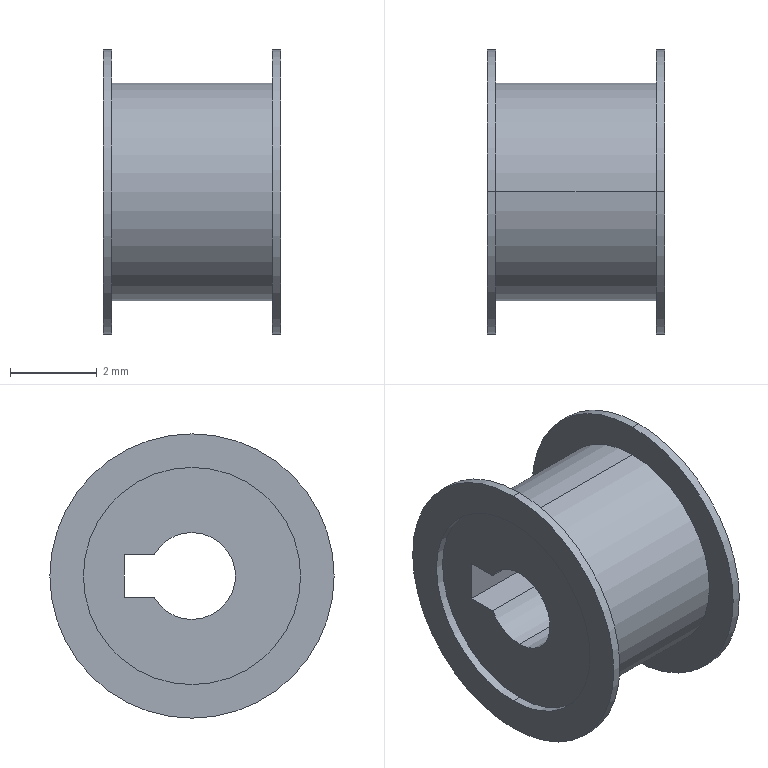Part | SolidWorks | features ICE 1, Revolution 1 | 3 solids | 22 faces | box 4.086 x 6.543 x 6.543 mm | volume 64.18 mm3 | cylinder 13 | plane 9 | commonest cylinder face diameters 5 x6 6.543 x4 2 x3
STEP:
#1=CARTESIAN_POINT('',(2.043,0.,3.271));
#2=VERTEX_POINT('',#1);
#3=CARTESIAN_POINT('',(2.043,0.,-3.271));
#4=VERTEX_POINT('',#3);
#5=CARTESIAN_POINT('',(2.043,0.,0.));
#6=DIRECTION('',(-1.,0.,0.));
#7=DIRECTION('',(0.,0.,1.));
#8=AXIS2_PLACEMENT_3D('',#5,#6,#7);
#9=CIRCLE('',#8,3.271);
#10=EDGE_CURVE('',#2,#4,#9,.T.);
#11=ORIENTED_EDGE('',*,*,#10,.T.);
#12=CARTESIAN_POINT('',(1.843,0.,-3.271));
#13=VERTEX_POINT('',#12);
#14=CARTESIAN_POINT('',(0.,0.,-3.271));
#15=DIRECTION('',(-1.,0.,0.));
#16=VECTOR('',#15,1000.);
#17=LINE('',#14,#16);
#18=EDGE_CURVE('',#4,#13,#17,.T.);
#19=ORIENTED_EDGE('',*,*,#18,.T.);
#20=CARTESIAN_POINT('',(1.843,0.,3.271));
#21=VERTEX_POINT('',#20);
#22=CARTESIAN_POINT('',(1.843,0.,0.));
#23=DIRECTION('',(-1.,0.,0.));
#24=DIRECTION('',(0.,0.,1.));
#25=AXIS2_PLACEMENT_3D('',#22,#23,#24);
#26=CIRCLE('',#25,3.271);
#27=EDGE_CURVE('',#21,#13,#26,.T.);
#28=ORIENTED_EDGE('',*,*,#27,.F.);
#29=CARTESIAN_POINT('',(0.,0.,3.271));
#30=DIRECTION('',(-1.,0.,0.));
#31=VECTOR('',#30,1000.);
#32=LINE('',#29,#31);
#33=EDGE_CURVE('',#2,#21,#32,.T.);
#34=ORIENTED_EDGE('',*,*,#33,.F.);
#35=EDGE_LOOP('',(#11,#19,#28,#34));
#36=FACE_OUTER_BOUND('',#35,.T.);
#37=CARTESIAN_POINT('',(0.,0.,0.));
#38=DIRECTION('',(-1.,0.,0.));
#39=DIRECTION('',(0.,0.,1.));
#40=AXIS2_PLACEMENT_3D('',#37,#38,#39);
#41=CYLINDRICAL_SURFACE('',#40,3.271);
#42=ADVANCED_FACE('',(#36),#41,.T.);
#43=CARTESIAN_POINT('',(2.043,0.,-2.5));
#44=VERTEX_POINT('',#43);
#45=CARTESIAN_POINT('',(2.043,0.,2.5));
#46=VERTEX_POINT('',#45);
#47=CARTESIAN_POINT('',(2.043,0.,0.));
#48=DIRECTION('',(-1.,0.,0.));
#49=DIRECTION('',(0.,0.,1.));
#50=AXIS2_PLACEMENT_3D('',#47,#48,#49);
#51=CIRCLE('',#50,2.5);
#52=EDGE_CURVE('',#44,#46,#51,.T.);
#53=ORIENTED_EDGE('',*,*,#52,.F.);
#54=CARTESIAN_POINT('',(1.843,0.,-2.5));
#55=VERTEX_POINT('',#54);
#56=CARTESIAN_POINT('',(0.,0.,-2.5));
#57=DIRECTION('',(-1.,0.,0.));
#58=VECTOR('',#57,1000.);
#59=LINE('',#56,#58);
#60=EDGE_CURVE('',#44,#55,#59,.T.);
#61=ORIENTED_EDGE('',*,*,#60,.T.);
#62=CARTESIAN_POINT('',(1.843,0.,2.5));
#63=VERTEX_POINT('',#62);
#64=CARTESIAN_POINT('',(1.843,0.,0.));
#65=DIRECTION('',(-1.,0.,0.));
#66=DIRECTION('',(0.,0.,1.));
#67=AXIS2_PLACEMENT_3D('',#64,#65,#66);
#68=CIRCLE('',#67,2.5);
#69=EDGE_CURVE('',#55,#63,#68,.T.);
#70=ORIENTED_EDGE('',*,*,#69,.T.);
#71=CARTESIAN_POINT('',(0.,0.,2.5));
#72=DIRECTION('',(-1.,0.,0.));
#73=VECTOR('',#72,1000.);
#74=LINE('',#71,#73);
#75=EDGE_CURVE('',#46,#63,#74,.T.);
#76=ORIENTED_EDGE('',*,*,#75,.F.);
#77=EDGE_LOOP('',(#53,#61,#70,#76));
#78=FACE_OUTER_BOUND('',#77,.T.);
#79=CARTESIAN_POINT('',(0.,0.,0.));
#80=DIRECTION('',(-1.,0.,0.));
#81=DIRECTION('',(0.,0.,1.));
#82=AXIS2_PLACEMENT_3D('',#79,#80,#81);
#83=CYLINDRICAL_SURFACE('',#82,2.5);
#84=ADVANCED_FACE('',(#78),#83,.F.);
#85=ORIENTED_EDGE('',*,*,#27,.T.);
#86=CARTESIAN_POINT('',(1.843,0.,0.));
#87=DIRECTION('',(-1.,0.,0.));
#88=DIRECTION('',(0.,0.,1.));
#89=AXIS2_PLACEMENT_3D('',#86,#87,#88);
#90=CIRCLE('',#89,3.271);
#91=EDGE_CURVE('',#13,#21,#90,.T.);
#92=ORIENTED_EDGE('',*,*,#91,.T.);
#93=EDGE_LOOP('',(#85,#92));
#94=FACE_OUTER_BOUND('',#93,.T.);
#95=CARTESIAN_POINT('',(1.843,0.,0.));
#96=DIRECTION('',(-1.,0.,0.));
#97=DIRECTION('',(0.,0.,1.));
#98=AXIS2_PLACEMENT_3D('',#95,#96,#97);
#99=CIRCLE('',#98,2.5);
#100=EDGE_CURVE('',#63,#55,#99,.T.);
#101=ORIENTED_EDGE('',*,*,#100,.F.);
#102=ORIENTED_EDGE('',*,*,#69,.F.);
#103=EDGE_LOOP('',(#101,#102));
#104=FACE_BOUND('',#103,.T.);
#105=CARTESIAN_POINT('',(1.843,0.,0.));
#106=DIRECTION('',(-1.,0.,0.));
#107=DIRECTION('',(0.,0.,1.));
#108=AXIS2_PLACEMENT_3D('',#105,#106,#107);
#109=PLANE('',#108);
#110=ADVANCED_FACE('',(#94,#104),#109,.T.);
#111=ORIENTED_EDGE('',*,*,#60,.F.);
#112=CARTESIAN_POINT('',(2.043,0.,0.));
#113=DIRECTION('',(-1.,0.,0.));
#114=DIRECTION('',(0.,0.,1.));
#115=AXIS2_PLACEMENT_3D('',#112,#113,#114);
#116=CIRCLE('',#115,2.5);
#117=EDGE_CURVE('',#46,#44,#116,.T.);
#118=ORIENTED_EDGE('',*,*,#117,.F.);
#119=ORIENTED_EDGE('',*,*,#75,.T.);
#120=ORIENTED_EDGE('',*,*,#100,.T.);
#121=EDGE_LOOP('',(#111,#118,#119,#120));
#122=FACE_OUTER_BOUND('',#121,.T.);
#123=CARTESIAN_POINT('',(0.,0.,0.));
#124=DIRECTION('',(-1.,0.,0.));
#125=DIRECTION('',(0.,0.,1.));
#126=AXIS2_PLACEMENT_3D('',#123,#124,#125);
#127=CYLINDRICAL_SURFACE('',#126,2.5);
#128=ADVANCED_FACE('',(#122),#127,.F.);
#129=ORIENTED_EDGE('',*,*,#10,.F.);
#130=CARTESIAN_POINT('',(2.043,0.,0.));
#131=DIRECTION('',(-1.,0.,0.));
#132=DIRECTION('',(0.,0.,1.));
#133=AXIS2_PLACEMENT_3D('',#130,#131,#132);
#134=CIRCLE('',#133,3.271);
#135=EDGE_CURVE('',#4,#2,#134,.T.);
#136=ORIENTED_EDGE('',*,*,#135,.F.);
#137=EDGE_LOOP('',(#129,#136));
#138=FACE_OUTER_BOUND('',#137,.T.);
#139=ORIENTED_EDGE('',*,*,#117,.T.);
#140=ORIENTED_EDGE('',*,*,#52,.T.);
#141=EDGE_LOOP('',(#139,#140));
#142=FACE_BOUND('',#141,.T.);
#143=CARTESIAN_POINT('',(2.043,0.,0.));
#144=DIRECTION('',(-1.,0.,0.));
#145=DIRECTION('',(0.,0.,1.));
#146=AXIS2_PLACEMENT_3D('',#143,#144,#145);
#147=PLANE('',#146);
#148=ADVANCED_FACE('',(#138,#142),#147,.F.);
#149=ORIENTED_EDGE('',*,*,#18,.F.);
#150=ORIENTED_EDGE('',*,*,#135,.T.);
#151=ORIENTED_EDGE('',*,*,#33,.T.);
#152=ORIENTED_EDGE('',*,*,#91,.F.);
#153=EDGE_LOOP('',(#149,#150,#151,#152));
#154=FACE_OUTER_BOUND('',#153,.T.);
#155=CARTESIAN_POINT('',(0.,0.,0.));
#156=DIRECTION('',(-1.,0.,0.));
#157=DIRECTION('',(0.,0.,1.));
#158=AXIS2_PLACEMENT_3D('',#155,#156,#157);
#159=CYLINDRICAL_SURFACE('',#158,3.271);
#160=ADVANCED_FACE('',(#154),#159,.T.);
#161=CLOSED_SHELL('',(#42,#84,#110,#128,#148,#160));
#162=MANIFOLD_SOLID_BREP('',#161);
#163=CARTESIAN_POINT('',(-1.843,0.,3.271));
#164=VERTEX_POINT('',#163);
#165=CARTESIAN_POINT('',(-1.843,0.,-3.271));
#166=VERTEX_POINT('',#165);
#167=CARTESIAN_POINT('',(-1.843,0.,0.));
#168=DIRECTION('',(-1.,0.,0.));
#169=DIRECTION('',(0.,0.,1.));
#170=AXIS2_PLACEMENT_3D('',#167,#168,#169);
#171=CIRCLE('',#170,3.271);
#172=EDGE_CURVE('',#164,#166,#171,.T.);
#173=ORIENTED_EDGE('',*,*,#172,.T.);
#174=CARTESIAN_POINT('',(-2.043,0.,-3.271));
#175=VERTEX_POINT('',#174);
#176=CARTESIAN_POINT('',(0.,0.,-3.271));
#177=DIRECTION('',(-1.,0.,0.));
#178=VECTOR('',#177,1000.);
#179=LINE('',#176,#178);
#180=EDGE_CURVE('',#166,#175,#179,.T.);
#181=ORIENTED_EDGE('',*,*,#180,.T.);
#182=CARTESIAN_POINT('',(-2.043,0.,3.271));
#183=VERTEX_POINT('',#182);
#184=CARTESIAN_POINT('',(-2.043,0.,0.));
#185=DIRECTION('',(-1.,0.,0.));
#186=DIRECTION('',(0.,0.,1.));
#187=AXIS2_PLACEMENT_3D('',#184,#185,#186);
#188=CIRCLE('',#187,3.271);
#189=EDGE_CURVE('',#183,#175,#188,.T.);
#190=ORIENTED_EDGE('',*,*,#189,.F.);
#191=CARTESIAN_POINT('',(0.,0.,3.271));
#192=DIRECTION('',(-1.,0.,0.));
#193=VECTOR('',#192,1000.);
#194=LINE('',#191,#193);
#195=EDGE_CURVE('',#164,#183,#194,.T.);
#196=ORIENTED_EDGE('',*,*,#195,.F.);
#197=EDGE_LOOP('',(#173,#181,#190,#196));
#198=FACE_OUTER_BOUND('',#197,.T.);
#199=CARTESIAN_POINT('',(0.,0.,0.));
#200=DIRECTION('',(-1.,0.,0.));
#201=DIRECTION('',(0.,0.,1.));
#202=AXIS2_PLACEMENT_3D('',#199,#200,#201);
#203=CYLINDRICAL_SURFACE('',#202,3.271);
#204=ADVANCED_FACE('',(#198),#203,.T.);
#205=CARTESIAN_POINT('',(-1.843,0.,-2.5));
#206=VERTEX_POINT('',#205);
#207=CARTESIAN_POINT('',(-1.843,0.,2.5));
#208=VERTEX_POINT('',#207);
#209=CARTESIAN_POINT('',(-1.843,0.,0.));
#210=DIRECTION('',(-1.,0.,0.));
#211=DIRECTION('',(0.,0.,1.));
#212=AXIS2_PLACEMENT_3D('',#209,#210,#211);
#213=CIRCLE('',#212,2.5);
#214=EDGE_CURVE('',#206,#208,#213,.T.);
#215=ORIENTED_EDGE('',*,*,#214,.F.);
#216=CARTESIAN_POINT('',(-2.043,0.,-2.5));
#217=VERTEX_POINT('',#216);
#218=CARTESIAN_POINT('',(0.,0.,-2.5));
#219=DIRECTION('',(-1.,0.,0.));
#220=VECTOR('',#219,1000.);
#221=LINE('',#218,#220);
#222=EDGE_CURVE('',#206,#217,#221,.T.);
#223=ORIENTED_EDGE('',*,*,#222,.T.);
#224=CARTESIAN_POINT('',(-2.043,0.,2.5));
#225=VERTEX_POINT('',#224);
#226=CARTESIAN_POINT('',(-2.043,0.,0.));
#227=DIRECTION('',(-1.,0.,0.));
#228=DIRECTION('',(0.,0.,1.));
#229=AXIS2_PLACEMENT_3D('',#226,#227,#228);
#230=CIRCLE('',#229,2.5);
#231=EDGE_CURVE('',#217,#225,#230,.T.);
#232=ORIENTED_EDGE('',*,*,#231,.T.);
#233=CARTESIAN_POINT('',(0.,0.,2.5));
#234=DIRECTION('',(-1.,0.,0.));
#235=VECTOR('',#234,1000.);
#236=LINE('',#233,#235);
#237=EDGE_CURVE('',#208,#225,#236,.T.);
#238=ORIENTED_EDGE('',*,*,#237,.F.);
#239=EDGE_LOOP('',(#215,#223,#232,#238));
#240=FACE_OUTER_BOUND('',#239,.T.);
#241=CARTESIAN_POINT('',(0.,0.,0.));
#242=DIRECTION('',(-1.,0.,0.));
#243=DIRECTION('',(0.,0.,1.));
#244=AXIS2_PLACEMENT_3D('',#241,#242,#243);
#245=CYLINDRICAL_SURFACE('',#244,2.5);
#246=ADVANCED_FACE('',(#240),#245,.F.);
#247=ORIENTED_EDGE('',*,*,#222,.F.);
#248=CARTESIAN_POINT('',(-1.843,0.,0.));
#249=DIRECTION('',(-1.,0.,0.));
#250=DIRECTION('',(0.,0.,1.));
#251=AXIS2_PLACEMENT_3D('',#248,#249,#250);
#252=CIRCLE('',#251,2.5);
#253=EDGE_CURVE('',#208,#206,#252,.T.);
#254=ORIENTED_EDGE('',*,*,#253,.F.);
#255=ORIENTED_EDGE('',*,*,#237,.T.);
#256=CARTESIAN_POINT('',(-2.043,0.,0.));
#257=DIRECTION('',(-1.,0.,0.));
#258=DIRECTION('',(0.,0.,1.));
#259=AXIS2_PLACEMENT_3D('',#256,#257,#258);
#260=CIRCLE('',#259,2.5);
#261=EDGE_CURVE('',#225,#217,#260,.T.);
#262=ORIENTED_EDGE('',*,*,#261,.T.);
#263=EDGE_LOOP('',(#247,#254,#255,#262));
#264=FACE_OUTER_BOUND('',#263,.T.);
#265=CARTESIAN_POINT('',(0.,0.,0.));
#266=DIRECTION('',(-1.,0.,0.));
#267=DIRECTION('',(0.,0.,1.));
#268=AXIS2_PLACEMENT_3D('',#265,#266,#267);
#269=CYLINDRICAL_SURFACE('',#268,2.5);
#270=ADVANCED_FACE('',(#264),#269,.F.);
#271=ORIENTED_EDGE('',*,*,#172,.F.);
#272=CARTESIAN_POINT('',(-1.843,0.,0.));
#273=DIRECTION('',(-1.,0.,0.));
#274=DIRECTION('',(0.,0.,1.));
#275=AXIS2_PLACEMENT_3D('',#272,#273,#274);
#276=CIRCLE('',#275,3.271);
#277=EDGE_CURVE('',#166,#164,#276,.T.);
#278=ORIENTED_EDGE('',*,*,#277,.F.);
#279=EDGE_LOOP('',(#271,#278));
#280=FACE_OUTER_BOUND('',#279,.T.);
#281=ORIENTED_EDGE('',*,*,#253,.T.);
#282=ORIENTED_EDGE('',*,*,#214,.T.);
#283=EDGE_LOOP('',(#281,#282));
#284=FACE_BOUND('',#283,.T.);
#285=CARTESIAN_POINT('',(-1.843,0.,0.));
#286=DIRECTION('',(-1.,0.,0.));
#287=DIRECTION('',(0.,0.,1.));
#288=AXIS2_PLACEMENT_3D('',#285,#286,#287);
#289=PLANE('',#288);
#290=ADVANCED_FACE('',(#280,#284),#289,.F.);
#291=ORIENTED_EDGE('',*,*,#180,.F.);
#292=ORIENTED_EDGE('',*,*,#277,.T.);
#293=ORIENTED_EDGE('',*,*,#195,.T.);
#294=CARTESIAN_POINT('',(-2.043,0.,0.));
#295=DIRECTION('',(-1.,0.,0.));
#296=DIRECTION('',(0.,0.,1.));
#297=AXIS2_PLACEMENT_3D('',#294,#295,#296);
#298=CIRCLE('',#297,3.271);
#299=EDGE_CURVE('',#175,#183,#298,.T.);
#300=ORIENTED_EDGE('',*,*,#299,.F.);
#301=EDGE_LOOP('',(#291,#292,#293,#300));
#302=FACE_OUTER_BOUND('',#301,.T.);
#303=CARTESIAN_POINT('',(0.,0.,0.));
#304=DIRECTION('',(-1.,0.,0.));
#305=DIRECTION('',(0.,0.,1.));
#306=AXIS2_PLACEMENT_3D('',#303,#304,#305);
#307=CYLINDRICAL_SURFACE('',#306,3.271);
#308=ADVANCED_FACE('',(#302),#307,.T.);
#309=ORIENTED_EDGE('',*,*,#189,.T.);
#310=ORIENTED_EDGE('',*,*,#299,.T.);
#311=EDGE_LOOP('',(#309,#310));
#312=FACE_OUTER_BOUND('',#311,.T.);
#313=ORIENTED_EDGE('',*,*,#261,.F.);
#314=ORIENTED_EDGE('',*,*,#231,.F.);
#315=EDGE_LOOP('',(#313,#314));
#316=FACE_BOUND('',#315,.T.);
#317=CARTESIAN_POINT('',(-2.043,0.,0.));
#318=DIRECTION('',(-1.,0.,0.));
#319=DIRECTION('',(0.,0.,1.));
#320=AXIS2_PLACEMENT_3D('',#317,#318,#319);
#321=PLANE('',#320);
#322=ADVANCED_FACE('',(#312,#316),#321,.T.);
#323=CLOSED_SHELL('',(#204,#246,#270,#290,#308,#322));
#324=MANIFOLD_SOLID_BREP('',#323);
#325=CARTESIAN_POINT('',(1.843,0.,2.5));
#326=VERTEX_POINT('',#325);
#327=CARTESIAN_POINT('',(1.843,0.,-2.5));
#328=VERTEX_POINT('',#327);
#329=CARTESIAN_POINT('',(1.843,0.,0.));
#330=DIRECTION('',(-1.,0.,0.));
#331=DIRECTION('',(0.,0.,1.));
#332=AXIS2_PLACEMENT_3D('',#329,#330,#331);
#333=CIRCLE('',#332,2.5);
#334=EDGE_CURVE('',#326,#328,#333,.T.);
#335=ORIENTED_EDGE('',*,*,#334,.T.);
#336=CARTESIAN_POINT('',(-1.843,0.,-2.5));
#337=VERTEX_POINT('',#336);
#338=CARTESIAN_POINT('',(0.,0.,-2.5));
#339=DIRECTION('',(-1.,0.,0.));
#340=VECTOR('',#339,1000.);
#341=LINE('',#338,#340);
#342=EDGE_CURVE('',#328,#337,#341,.T.);
#343=ORIENTED_EDGE('',*,*,#342,.T.);
#344=CARTESIAN_POINT('',(-1.843,0.,2.5));
#345=VERTEX_POINT('',#344);
#346=CARTESIAN_POINT('',(-1.843,0.,0.));
#347=DIRECTION('',(-1.,0.,0.));
#348=DIRECTION('',(0.,0.,1.));
#349=AXIS2_PLACEMENT_3D('',#346,#347,#348);
#350=CIRCLE('',#349,2.5);
#351=EDGE_CURVE('',#345,#337,#350,.T.);
#352=ORIENTED_EDGE('',*,*,#351,.F.);
#353=CARTESIAN_POINT('',(0.,0.,2.5));
#354=DIRECTION('',(-1.,0.,0.));
#355=VECTOR('',#354,1000.);
#356=LINE('',#353,#355);
#357=EDGE_CURVE('',#326,#345,#356,.T.);
#358=ORIENTED_EDGE('',*,*,#357,.F.);
#359=EDGE_LOOP('',(#335,#343,#352,#358));
#360=FACE_OUTER_BOUND('',#359,.T.);
#361=CARTESIAN_POINT('',(0.,0.,0.));
#362=DIRECTION('',(-1.,0.,0.));
#363=DIRECTION('',(0.,0.,1.));
#364=AXIS2_PLACEMENT_3D('',#361,#362,#363);
#365=CYLINDRICAL_SURFACE('',#364,2.5);
#366=ADVANCED_FACE('',(#360),#365,.T.);
#367=CARTESIAN_POINT('',(1.843,0.,-1.));
#368=VERTEX_POINT('',#367);
#369=CARTESIAN_POINT('',(1.843,0.,1.));
#370=VERTEX_POINT('',#369);
#371=CARTESIAN_POINT('',(1.843,0.,0.));
#372=DIRECTION('',(-1.,0.,0.));
#373=DIRECTION('',(0.,0.,1.));
#374=AXIS2_PLACEMENT_3D('',#371,#372,#373);
#375=CIRCLE('',#374,1.);
#376=EDGE_CURVE('',#368,#370,#375,.T.);
#377=ORIENTED_EDGE('',*,*,#376,.F.);
#378=CARTESIAN_POINT('',(-1.843,0.,-1.));
#379=VERTEX_POINT('',#378);
#380=CARTESIAN_POINT('',(0.,0.,-1.));
#381=DIRECTION('',(-1.,0.,0.));
#382=VECTOR('',#381,1000.);
#383=LINE('',#380,#382);
#384=EDGE_CURVE('',#368,#379,#383,.T.);
#385=ORIENTED_EDGE('',*,*,#384,.T.);
#386=CARTESIAN_POINT('',(-1.843,0.,1.));
#387=VERTEX_POINT('',#386);
#388=CARTESIAN_POINT('',(-1.843,0.,0.));
#389=DIRECTION('',(-1.,0.,0.));
#390=DIRECTION('',(0.,0.,1.));
#391=AXIS2_PLACEMENT_3D('',#388,#389,#390);
#392=CIRCLE('',#391,1.);
#393=EDGE_CURVE('',#379,#387,#392,.T.);
#394=ORIENTED_EDGE('',*,*,#393,.T.);
#395=CARTESIAN_POINT('',(0.,0.,1.));
#396=DIRECTION('',(-1.,0.,0.));
#397=VECTOR('',#396,1000.);
#398=LINE('',#395,#397);
#399=EDGE_CURVE('',#370,#387,#398,.T.);
#400=ORIENTED_EDGE('',*,*,#399,.F.);
#401=EDGE_LOOP('',(#377,#385,#394,#400));
#402=FACE_OUTER_BOUND('',#401,.T.);
#403=CARTESIAN_POINT('',(0.,0.,0.));
#404=DIRECTION('',(-1.,0.,0.));
#405=DIRECTION('',(0.,0.,1.));
#406=AXIS2_PLACEMENT_3D('',#403,#404,#405);
#407=CYLINDRICAL_SURFACE('',#406,1.);
#408=ADVANCED_FACE('',(#402),#407,.F.);
#409=CARTESIAN_POINT('',(1.843,0.8691,0.4947));
#410=VERTEX_POINT('',#409);
#411=CARTESIAN_POINT('',(1.843,0.,0.));
#412=DIRECTION('',(-1.,0.,0.));
#413=DIRECTION('',(0.,0.,1.));
#414=AXIS2_PLACEMENT_3D('',#411,#412,#413);
#415=CIRCLE('',#414,1.);
#416=EDGE_CURVE('',#370,#410,#415,.T.);
#417=ORIENTED_EDGE('',*,*,#416,.F.);
#418=ORIENTED_EDGE('',*,*,#399,.T.);
#419=CARTESIAN_POINT('',(-1.843,0.8691,0.4947));
#420=VERTEX_POINT('',#419);
#421=CARTESIAN_POINT('',(-1.843,0.,0.));
#422=DIRECTION('',(-1.,0.,0.));
#423=DIRECTION('',(0.,0.,1.));
#424=AXIS2_PLACEMENT_3D('',#421,#422,#423);
#425=CIRCLE('',#424,1.);
#426=EDGE_CURVE('',#387,#420,#425,.T.);
#427=ORIENTED_EDGE('',*,*,#426,.T.);
#428=CARTESIAN_POINT('',(8.157,0.8691,0.4947));
#429=DIRECTION('',(-1.,0.,0.));
#430=VECTOR('',#429,1000.);
#431=LINE('',#428,#430);
#432=EDGE_CURVE('',#410,#420,#431,.T.);
#433=ORIENTED_EDGE('',*,*,#432,.F.);
#434=EDGE_LOOP('',(#417,#418,#427,#433));
#435=FACE_OUTER_BOUND('',#434,.T.);
#436=CARTESIAN_POINT('',(0.,0.,0.));
#437=DIRECTION('',(-1.,0.,0.));
#438=DIRECTION('',(0.,0.,1.));
#439=AXIS2_PLACEMENT_3D('',#436,#437,#438);
#440=CYLINDRICAL_SURFACE('',#439,1.);
#441=ADVANCED_FACE('',(#435),#440,.F.);
#442=ORIENTED_EDGE('',*,*,#351,.T.);
#443=CARTESIAN_POINT('',(-1.843,0.,0.));
#444=DIRECTION('',(-1.,0.,0.));
#445=DIRECTION('',(0.,0.,1.));
#446=AXIS2_PLACEMENT_3D('',#443,#444,#445);
#447=CIRCLE('',#446,2.5);
#448=EDGE_CURVE('',#337,#345,#447,.T.);
#449=ORIENTED_EDGE('',*,*,#448,.T.);
#450=EDGE_LOOP('',(#442,#449));
#451=FACE_OUTER_BOUND('',#450,.T.);
#452=CARTESIAN_POINT('',(-1.843,0.8691,-0.4947));
#453=VERTEX_POINT('',#452);
#454=CARTESIAN_POINT('',(-1.843,0.,0.));
#455=DIRECTION('',(-1.,0.,0.));
#456=DIRECTION('',(0.,0.,1.));
#457=AXIS2_PLACEMENT_3D('',#454,#455,#456);
#458=CIRCLE('',#457,1.);
#459=EDGE_CURVE('',#453,#379,#458,.T.);
#460=ORIENTED_EDGE('',*,*,#459,.F.);
#461=CARTESIAN_POINT('',(-1.843,1.562,-0.4947));
#462=VERTEX_POINT('',#461);
#463=CARTESIAN_POINT('',(-1.843,0.,-0.4947));
#464=DIRECTION('',(0.,1.,0.));
#465=VECTOR('',#464,1000.);
#466=LINE('',#463,#465);
#467=EDGE_CURVE('',#453,#462,#466,.T.);
#468=ORIENTED_EDGE('',*,*,#467,.T.);
#469=CARTESIAN_POINT('',(-1.843,1.562,0.4947));
#470=VERTEX_POINT('',#469);
#471=CARTESIAN_POINT('',(-1.843,1.562,0.));
#472=DIRECTION('',(0.,0.,1.));
#473=VECTOR('',#472,1000.);
#474=LINE('',#471,#473);
#475=EDGE_CURVE('',#462,#470,#474,.T.);
#476=ORIENTED_EDGE('',*,*,#475,.T.);
#477=CARTESIAN_POINT('',(-1.843,0.,0.4947));
#478=DIRECTION('',(0.,1.,0.));
#479=VECTOR('',#478,1000.);
#480=LINE('',#477,#479);
#481=EDGE_CURVE('',#420,#470,#480,.T.);
#482=ORIENTED_EDGE('',*,*,#481,.F.);
#483=ORIENTED_EDGE('',*,*,#426,.F.);
#484=ORIENTED_EDGE('',*,*,#393,.F.);
#485=EDGE_LOOP('',(#460,#468,#476,#482,#483,#484));
#486=FACE_BOUND('',#485,.T.);
#487=CARTESIAN_POINT('',(-1.843,0.,0.));
#488=DIRECTION('',(-1.,0.,0.));
#489=DIRECTION('',(0.,0.,1.));
#490=AXIS2_PLACEMENT_3D('',#487,#488,#489);
#491=PLANE('',#490);
#492=ADVANCED_FACE('',(#451,#486),#491,.T.);
#493=ORIENTED_EDGE('',*,*,#384,.F.);
#494=CARTESIAN_POINT('',(1.843,0.8691,-0.4947));
#495=VERTEX_POINT('',#494);
#496=CARTESIAN_POINT('',(1.843,0.,0.));
#497=DIRECTION('',(-1.,0.,0.));
#498=DIRECTION('',(0.,0.,1.));
#499=AXIS2_PLACEMENT_3D('',#496,#497,#498);
#500=CIRCLE('',#499,1.);
#501=EDGE_CURVE('',#495,#368,#500,.T.);
#502=ORIENTED_EDGE('',*,*,#501,.F.);
#503=CARTESIAN_POINT('',(8.157,0.8691,-0.4947));
#504=DIRECTION('',(-1.,0.,0.));
#505=VECTOR('',#504,1000.);
#506=LINE('',#503,#505);
#507=EDGE_CURVE('',#495,#453,#506,.T.);
#508=ORIENTED_EDGE('',*,*,#507,.T.);
#509=ORIENTED_EDGE('',*,*,#459,.T.);
#510=EDGE_LOOP('',(#493,#502,#508,#509));
#511=FACE_OUTER_BOUND('',#510,.T.);
#512=CARTESIAN_POINT('',(0.,0.,0.));
#513=DIRECTION('',(-1.,0.,0.));
#514=DIRECTION('',(0.,0.,1.));
#515=AXIS2_PLACEMENT_3D('',#512,#513,#514);
#516=CYLINDRICAL_SURFACE('',#515,1.);
#517=ADVANCED_FACE('',(#511),#516,.F.);
#518=ORIENTED_EDGE('',*,*,#334,.F.);
#519=CARTESIAN_POINT('',(1.843,0.,0.));
#520=DIRECTION('',(-1.,0.,0.));
#521=DIRECTION('',(0.,0.,1.));
#522=AXIS2_PLACEMENT_3D('',#519,#520,#521);
#523=CIRCLE('',#522,2.5);
#524=EDGE_CURVE('',#328,#326,#523,.T.);
#525=ORIENTED_EDGE('',*,*,#524,.F.);
#526=EDGE_LOOP('',(#518,#525));
#527=FACE_OUTER_BOUND('',#526,.T.);
#528=CARTESIAN_POINT('',(1.843,1.562,-0.4947));
#529=VERTEX_POINT('',#528);
#530=CARTESIAN_POINT('',(1.843,0.,-0.4947));
#531=DIRECTION('',(0.,1.,0.));
#532=VECTOR('',#531,1000.);
#533=LINE('',#530,#532);
#534=EDGE_CURVE('',#495,#529,#533,.T.);
#535=ORIENTED_EDGE('',*,*,#534,.F.);
#536=ORIENTED_EDGE('',*,*,#501,.T.);
#537=ORIENTED_EDGE('',*,*,#376,.T.);
#538=ORIENTED_EDGE('',*,*,#416,.T.);
#539=CARTESIAN_POINT('',(1.843,1.562,0.4947));
#540=VERTEX_POINT('',#539);
#541=CARTESIAN_POINT('',(1.843,0.,0.4947));
#542=DIRECTION('',(0.,1.,0.));
#543=VECTOR('',#542,1000.);
#544=LINE('',#541,#543);
#545=EDGE_CURVE('',#410,#540,#544,.T.);
#546=ORIENTED_EDGE('',*,*,#545,.T.);
#547=CARTESIAN_POINT('',(1.843,1.562,0.));
#548=DIRECTION('',(0.,0.,1.));
#549=VECTOR('',#548,1000.);
#550=LINE('',#547,#549);
#551=EDGE_CURVE('',#529,#540,#550,.T.);
#552=ORIENTED_EDGE('',*,*,#551,.F.);
#553=EDGE_LOOP('',(#535,#536,#537,#538,#546,#552));
#554=FACE_BOUND('',#553,.T.);
#555=CARTESIAN_POINT('',(1.843,0.,0.));
#556=DIRECTION('',(-1.,0.,0.));
#557=DIRECTION('',(0.,0.,1.));
#558=AXIS2_PLACEMENT_3D('',#555,#556,#557);
#559=PLANE('',#558);
#560=ADVANCED_FACE('',(#527,#554),#559,.F.);
#561=ORIENTED_EDGE('',*,*,#342,.F.);
#562=ORIENTED_EDGE('',*,*,#524,.T.);
#563=ORIENTED_EDGE('',*,*,#357,.T.);
#564=ORIENTED_EDGE('',*,*,#448,.F.);
#565=EDGE_LOOP('',(#561,#562,#563,#564));
#566=FACE_OUTER_BOUND('',#565,.T.);
#567=CARTESIAN_POINT('',(0.,0.,0.));
#568=DIRECTION('',(-1.,0.,0.));
#569=DIRECTION('',(0.,0.,1.));
#570=AXIS2_PLACEMENT_3D('',#567,#568,#569);
#571=CYLINDRICAL_SURFACE('',#570,2.5);
#572=ADVANCED_FACE('',(#566),#571,.T.);
#573=ORIENTED_EDGE('',*,*,#534,.T.);
#574=CARTESIAN_POINT('',(8.157,1.562,-0.4947));
#575=DIRECTION('',(-1.,0.,0.));
#576=VECTOR('',#575,1000.);
#577=LINE('',#574,#576);
#578=EDGE_CURVE('',#529,#462,#577,.T.);
#579=ORIENTED_EDGE('',*,*,#578,.T.);
#580=ORIENTED_EDGE('',*,*,#467,.F.);
#581=ORIENTED_EDGE('',*,*,#507,.F.);
#582=EDGE_LOOP('',(#573,#579,#580,#581));
#583=FACE_OUTER_BOUND('',#582,.T.);
#584=CARTESIAN_POINT('',(8.157,0.,-0.4947));
#585=DIRECTION('',(0.,0.,1.));
#586=DIRECTION('',(1.,0.,0.));
#587=AXIS2_PLACEMENT_3D('',#584,#585,#586);
#588=PLANE('',#587);
#589=ADVANCED_FACE('',(#583),#588,.T.);
#590=ORIENTED_EDGE('',*,*,#551,.T.);
#591=CARTESIAN_POINT('',(8.157,1.562,0.4947));
#592=DIRECTION('',(-1.,0.,0.));
#593=VECTOR('',#592,1000.);
#594=LINE('',#591,#593);
#595=EDGE_CURVE('',#540,#470,#594,.T.);
#596=ORIENTED_EDGE('',*,*,#595,.T.);
#597=ORIENTED_EDGE('',*,*,#475,.F.);
#598=ORIENTED_EDGE('',*,*,#578,.F.);
#599=EDGE_LOOP('',(#590,#596,#597,#598));
#600=FACE_OUTER_BOUND('',#599,.T.);
#601=CARTESIAN_POINT('',(8.157,1.562,0.));
#602=DIRECTION('',(0.,-1.,0.));
#603=DIRECTION('',(0.,0.,-1.));
#604=AXIS2_PLACEMENT_3D('',#601,#602,#603);
#605=PLANE('',#604);
#606=ADVANCED_FACE('',(#600),#605,.T.);
#607=ORIENTED_EDGE('',*,*,#432,.T.);
#608=ORIENTED_EDGE('',*,*,#481,.T.);
#609=ORIENTED_EDGE('',*,*,#595,.F.);
#610=ORIENTED_EDGE('',*,*,#545,.F.);
#611=EDGE_LOOP('',(#607,#608,#609,#610));
#612=FACE_OUTER_BOUND('',#611,.T.);
#613=CARTESIAN_POINT('',(8.157,0.,0.4947));
#614=DIRECTION('',(0.,0.,1.));
#615=DIRECTION('',(1.,0.,0.));
#616=AXIS2_PLACEMENT_3D('',#613,#614,#615);
#617=PLANE('',#616);
#618=ADVANCED_FACE('',(#612),#617,.F.);
#619=CLOSED_SHELL('',(#366,#408,#441,#492,#517,#560,#572,#589,#606,#618));
#620=MANIFOLD_SOLID_BREP('',#619);
#621=CARTESIAN_POINT('',(0.,0.,0.));
#622=DIRECTION('',(0.,0.,1.));
#623=DIRECTION('',(1.,0.,0.));
#624=AXIS2_PLACEMENT_3D('',#621,#622,#623);
#625=(LENGTH_UNIT()NAMED_UNIT(*)SI_UNIT(.MILLI.,.METRE.));
#626=UNCERTAINTY_MEASURE_WITH_UNIT(LENGTH_MEASURE(0.00001),#625,'','');
#627=(NAMED_UNIT(*)PLANE_ANGLE_UNIT()SI_UNIT($,.RADIAN.));
#628=(NAMED_UNIT(*)SI_UNIT($,.STERADIAN.)SOLID_ANGLE_UNIT());
#629=(GEOMETRIC_REPRESENTATION_CONTEXT(3)GLOBAL_UNCERTAINTY_ASSIGNED_CONTEXT((#626))GLOBAL_UNIT_ASSIGNED_CONTEXT((#625,#627,#628))REPRESENTATION_CONTEXT('',''));
#630=ADVANCED_BREP_SHAPE_REPRESENTATION('',(#162,#324,#620,#624),#629);